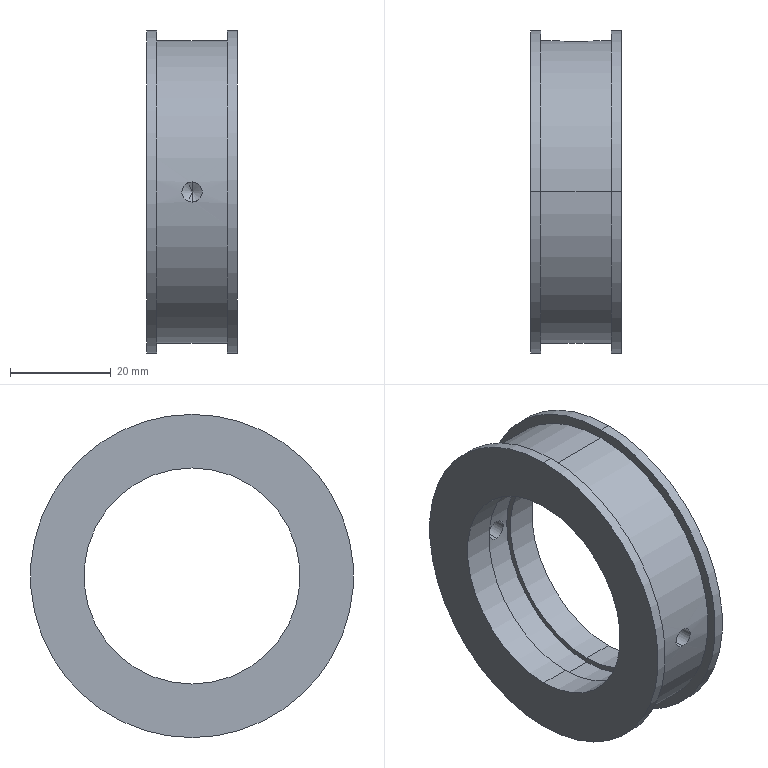Part | SolidWorks | features HoleWzd 3, Fillet 2, Revolution 1 | 1 solid | 31 faces | box 18 x 64 x 64 mm | volume 25534 mm3 | cylinder 18 | plane 7 | torus 2 | spline 2 | cone 2 | commonest cylinder face diameters 4 x4 42.8 x4 64 x4 7.5 x2 44.8 x2 60 x2
STEP:
#1=CARTESIAN_POINT('',(0.6103,28.8,3.75));
#2=VERTEX_POINT('',#1);
#3=CARTESIAN_POINT('',(0.6103,28.8,-3.75));
#4=VERTEX_POINT('',#3);
#5=CARTESIAN_POINT('',(0.6103,28.8,0.));
#6=DIRECTION('',(0.,-1.,0.));
#7=DIRECTION('',(0.,0.,-1.));
#8=AXIS2_PLACEMENT_3D('',#5,#6,#7);
#9=CIRCLE('',#8,3.75);
#10=EDGE_CURVE('',#2,#4,#9,.T.);
#11=ORIENTED_EDGE('',*,*,#10,.F.);
#12=CARTESIAN_POINT('',(0.6103,28.5,3.45));
#13=VERTEX_POINT('',#12);
#14=CARTESIAN_POINT('',(0.6103,28.8,3.45));
#15=DIRECTION('',(1.,0.,0.));
#16=DIRECTION('',(0.,0.,-1.));
#17=AXIS2_PLACEMENT_3D('',#14,#15,#16);
#18=CIRCLE('',#17,0.3);
#19=EDGE_CURVE('',#2,#13,#18,.T.);
#20=ORIENTED_EDGE('',*,*,#19,.T.);
#21=CARTESIAN_POINT('',(0.6103,28.5,-3.45));
#22=VERTEX_POINT('',#21);
#23=CARTESIAN_POINT('',(0.6103,28.5,0.));
#24=DIRECTION('',(0.,1.,0.));
#25=DIRECTION('',(0.,0.,-1.));
#26=AXIS2_PLACEMENT_3D('',#23,#24,#25);
#27=CIRCLE('',#26,3.45);
#28=EDGE_CURVE('',#22,#13,#27,.T.);
#29=ORIENTED_EDGE('',*,*,#28,.F.);
#30=CARTESIAN_POINT('',(0.6103,28.8,-3.45));
#31=DIRECTION('',(-1.,0.,0.));
#32=DIRECTION('',(0.,0.,1.));
#33=AXIS2_PLACEMENT_3D('',#30,#31,#32);
#34=CIRCLE('',#33,0.3);
#35=EDGE_CURVE('',#4,#22,#34,.T.);
#36=ORIENTED_EDGE('',*,*,#35,.F.);
#37=EDGE_LOOP('',(#11,#20,#29,#36));
#38=FACE_OUTER_BOUND('',#37,.T.);
#39=CARTESIAN_POINT('',(0.6103,28.8,0.));
#40=DIRECTION('',(0.,-1.,0.));
#41=DIRECTION('',(0.,0.,-1.));
#42=AXIS2_PLACEMENT_3D('',#39,#40,#41);
#43=TOROIDAL_SURFACE('',#42,3.45,0.3);
#44=ADVANCED_FACE('',(#38),#43,.F.);
#45=CARTESIAN_POINT('',(-0.2424,29.551,-3.652));
#46=VERTEX_POINT('',#45);
#47=CARTESIAN_POINT('',(0.6103,29.537,3.75));
#48=VERTEX_POINT('',#47);
#49=CARTESIAN_POINT('',(-0.2424,29.551,-3.652));
#50=CARTESIAN_POINT('',(-0.4646,29.558,-3.6));
#51=CARTESIAN_POINT('',(-0.6839,29.568,-3.527));
#52=CARTESIAN_POINT('',(-1.101,29.591,-3.345));
#53=CARTESIAN_POINT('',(-1.299,29.605,-3.236));
#54=CARTESIAN_POINT('',(-1.675,29.634,-2.982));
#55=CARTESIAN_POINT('',(-1.854,29.65,-2.836));
#56=CARTESIAN_POINT('',(-2.178,29.682,-2.518));
#57=CARTESIAN_POINT('',(-2.324,29.698,-2.346));
#58=CARTESIAN_POINT('',(-2.586,29.728,-1.974));
#59=CARTESIAN_POINT('',(-2.701,29.742,-1.774));
#60=CARTESIAN_POINT('',(-2.891,29.766,-1.363));
#61=CARTESIAN_POINT('',(-2.967,29.776,-1.149));
#62=CARTESIAN_POINT('',(-3.08,29.792,-0.7059));
#63=CARTESIAN_POINT('',(-3.116,29.797,-0.479));
#64=CARTESIAN_POINT('',(-3.146,29.801,-0.02683));
#65=CARTESIAN_POINT('',(-3.141,29.8,0.2003));
#66=CARTESIAN_POINT('',(-3.089,29.793,0.6567));
#67=CARTESIAN_POINT('',(-3.042,29.786,0.8794));
#68=CARTESIAN_POINT('',(-2.91,29.769,1.312));
#69=CARTESIAN_POINT('',(-2.823,29.757,1.524));
#70=CARTESIAN_POINT('',(-2.613,29.731,1.93));
#71=CARTESIAN_POINT('',(-2.491,29.717,2.121));
#72=CARTESIAN_POINT('',(-2.213,29.686,2.478));
#73=CARTESIAN_POINT('',(-2.056,29.67,2.647));
#74=CARTESIAN_POINT('',(-1.716,29.638,2.95));
#75=CARTESIAN_POINT('',(-1.534,29.623,3.084));
#76=CARTESIAN_POINT('',(-1.147,29.594,3.32));
#77=CARTESIAN_POINT('',(-0.9399,29.581,3.422));
#78=CARTESIAN_POINT('',(-0.5152,29.56,3.584));
#79=CARTESIAN_POINT('',(-0.2972,29.552,3.646));
#80=CARTESIAN_POINT('',(0.1503,29.54,3.729));
#81=CARTESIAN_POINT('',(0.3805,29.537,3.75));
#82=CARTESIAN_POINT('',(0.6103,29.537,3.75));
#83=B_SPLINE_CURVE_WITH_KNOTS('',3,(#49,#50,#51,#52,#53,#54,#55,#56,#57,#58,#59,#60,#61,#62,#63,#64,#65,#66,#67,#68,#69,#70,#71,#72,#73,#74,#75,#76,#77,#78,#79,#80,#81,#82),.UNSPECIFIED.,.F.,.F.,(4,2,2,2,2,2,2,2,2,2,2,2,2,2,2,2,4),(0.01269,0.01337,0.01406,0.01474,0.01543,0.01611,0.0168,0.01748,0.01817,0.01885,0.01954,0.02022,0.02091,0.02159,0.02228,0.02296,0.02365),.UNSPECIFIED.);
#84=EDGE_CURVE('',#46,#48,#83,.T.);
#85=ORIENTED_EDGE('',*,*,#84,.F.);
#86=CARTESIAN_POINT('',(-0.2879,29.749,-3.872));
#87=VERTEX_POINT('',#86);
#88=CARTESIAN_POINT('',(-0.2879,29.551,-3.847));
#89=DIRECTION('',(-0.9734,0.02959,0.2273));
#90=DIRECTION('',(0.2274,0.,0.9738));
#91=AXIS2_PLACEMENT_3D('',#88,#89,#90);
#92=CIRCLE('',#91,0.2);
#93=EDGE_CURVE('',#46,#87,#92,.T.);
#94=ORIENTED_EDGE('',*,*,#93,.T.);
#95=CARTESIAN_POINT('',(1.509,29.749,3.872));
#96=VERTEX_POINT('',#95);
#97=CARTESIAN_POINT('',(1.509,29.749,3.872));
#98=CARTESIAN_POINT('',(1.254,29.741,3.932));
#99=CARTESIAN_POINT('',(0.9958,29.737,3.966));
#100=CARTESIAN_POINT('',(0.4738,29.734,3.983));
#101=CARTESIAN_POINT('',(0.2098,29.737,3.965));
#102=CARTESIAN_POINT('',(-0.3023,29.748,3.878));
#103=CARTESIAN_POINT('',(-0.5513,29.757,3.81));
#104=CARTESIAN_POINT('',(-1.035,29.78,3.624));
#105=CARTESIAN_POINT('',(-1.271,29.795,3.506));
#106=CARTESIAN_POINT('',(-1.707,29.826,3.231));
#107=CARTESIAN_POINT('',(-1.911,29.843,3.072));
#108=CARTESIAN_POINT('',(-2.289,29.878,2.714));
#109=CARTESIAN_POINT('',(-2.459,29.895,2.517));
#110=CARTESIAN_POINT('',(-2.756,29.927,2.096));
#111=CARTESIAN_POINT('',(-2.886,29.943,1.869));
#112=CARTESIAN_POINT('',(-3.098,29.969,1.394));
#113=CARTESIAN_POINT('',(-3.18,29.979,1.149));
#114=CARTESIAN_POINT('',(-3.296,29.994,0.6447));
#115=CARTESIAN_POINT('',(-3.33,29.999,0.3829));
#116=CARTESIAN_POINT('',(-3.346,30.001,-0.135));
#117=CARTESIAN_POINT('',(-3.329,29.999,-0.3927));
#118=CARTESIAN_POINT('',(-3.245,29.987,-0.9056));
#119=CARTESIAN_POINT('',(-3.177,29.979,-1.16));
#120=CARTESIAN_POINT('',(-2.996,29.956,-1.643));
#121=CARTESIAN_POINT('',(-2.882,29.942,-1.876));
#122=CARTESIAN_POINT('',(-2.608,29.911,-2.321));
#123=CARTESIAN_POINT('',(-2.451,29.894,-2.526));
#124=CARTESIAN_POINT('',(-2.1,29.86,-2.904));
#125=CARTESIAN_POINT('',(-1.904,29.842,-3.078));
#126=CARTESIAN_POINT('',(-1.484,29.809,-3.382));
#127=CARTESIAN_POINT('',(-1.261,29.794,-3.512));
#128=CARTESIAN_POINT('',(-0.7903,29.768,-3.727));
#129=CARTESIAN_POINT('',(-0.5411,29.757,-3.813));
#130=CARTESIAN_POINT('',(-0.2879,29.749,-3.872));
#131=B_SPLINE_CURVE_WITH_KNOTS('',3,(#97,#98,#99,#100,#101,#102,#103,#104,#105,#106,#107,#108,#109,#110,#111,#112,#113,#114,#115,#116,#117,#118,#119,#120,#121,#122,#123,#124,#125,#126,#127,#128,#129,#130),.UNSPECIFIED.,.F.,.F.,(4,2,2,2,2,2,2,2,2,2,2,2,2,2,2,2,4),(0.02421,0.025,0.02578,0.02657,0.02735,0.02814,0.02892,0.02971,0.03049,0.03128,0.03206,0.03285,0.03363,0.03442,0.0352,0.03599,0.03677),.UNSPECIFIED.);
#132=EDGE_CURVE('',#96,#87,#131,.T.);
#133=ORIENTED_EDGE('',*,*,#132,.F.);
#134=CARTESIAN_POINT('',(1.463,29.551,3.652));
#135=VERTEX_POINT('',#134);
#136=CARTESIAN_POINT('',(1.509,29.551,3.846));
#137=DIRECTION('',(0.9734,0.02959,-0.2273));
#138=DIRECTION('',(-0.2274,0.,-0.9738));
#139=AXIS2_PLACEMENT_3D('',#136,#137,#138);
#140=CIRCLE('',#139,0.2);
#141=EDGE_CURVE('',#135,#96,#140,.T.);
#142=ORIENTED_EDGE('',*,*,#141,.F.);
#143=CARTESIAN_POINT('',(0.6103,29.537,3.75));
#144=CARTESIAN_POINT('',(0.7544,29.537,3.75));
#145=CARTESIAN_POINT('',(1.041,29.539,3.733));
#146=CARTESIAN_POINT('',(1.323,29.546,3.684));
#147=CARTESIAN_POINT('',(1.463,29.551,3.652));
#148=B_SPLINE_CURVE_WITH_KNOTS('',3,(#143,#144,#145,#146,#147),.UNSPECIFIED.,.F.,.F.,(4,1,4),(0.,0.0004293,0.0008586),.UNSPECIFIED.);
#149=EDGE_CURVE('',#48,#135,#148,.T.);
#150=ORIENTED_EDGE('',*,*,#149,.F.);
#151=EDGE_LOOP('',(#85,#94,#133,#142,#150));
#152=FACE_OUTER_BOUND('',#151,.T.);
#153=CARTESIAN_POINT('',(1.463,29.551,3.652));
#154=CARTESIAN_POINT('',(1.457,29.778,3.653));
#155=CARTESIAN_POINT('',(1.509,29.749,3.872));
#156=CARTESIAN_POINT('',(1.222,29.543,3.708));
#157=CARTESIAN_POINT('',(1.216,29.771,3.709));
#158=CARTESIAN_POINT('',(1.254,29.741,3.932));
#159=CARTESIAN_POINT('',(0.9788,29.538,3.74));
#160=CARTESIAN_POINT('',(0.9757,29.767,3.74));
#161=CARTESIAN_POINT('',(0.9985,29.737,3.966));
#162=CARTESIAN_POINT('',(0.49,29.536,3.756));
#163=CARTESIAN_POINT('',(0.4909,29.765,3.756));
#164=CARTESIAN_POINT('',(0.4835,29.734,3.983));
#165=CARTESIAN_POINT('',(0.2413,29.539,3.74));
#166=CARTESIAN_POINT('',(0.2448,29.767,3.74));
#167=CARTESIAN_POINT('',(0.2217,29.737,3.966));
#168=CARTESIAN_POINT('',(-0.2441,29.55,3.66));
#169=CARTESIAN_POINT('',(-0.237,29.777,3.661));
#170=CARTESIAN_POINT('',(-0.2896,29.748,3.881));
#171=CARTESIAN_POINT('',(-0.4801,29.558,3.596));
#172=CARTESIAN_POINT('',(-0.4712,29.784,3.599));
#173=CARTESIAN_POINT('',(-0.5383,29.757,3.814));
#174=CARTESIAN_POINT('',(-0.9391,29.581,3.424));
#175=CARTESIAN_POINT('',(-0.928,29.804,3.429));
#176=CARTESIAN_POINT('',(-1.022,29.78,3.631));
#177=CARTESIAN_POINT('',(-1.163,29.595,3.313));
#178=CARTESIAN_POINT('',(-1.151,29.817,3.32));
#179=CARTESIAN_POINT('',(-1.257,29.794,3.513));
#180=CARTESIAN_POINT('',(-1.578,29.626,3.055));
#181=CARTESIAN_POINT('',(-1.566,29.844,3.064));
#182=CARTESIAN_POINT('',(-1.695,29.825,3.24));
#183=CARTESIAN_POINT('',(-1.772,29.643,2.907));
#184=CARTESIAN_POINT('',(-1.76,29.859,2.916));
#185=CARTESIAN_POINT('',(-1.899,29.842,3.082));
#186=CARTESIAN_POINT('',(-2.132,29.677,2.57));
#187=CARTESIAN_POINT('',(-2.121,29.89,2.581));
#188=CARTESIAN_POINT('',(-2.278,29.877,2.725));
#189=CARTESIAN_POINT('',(-2.294,29.695,2.384));
#190=CARTESIAN_POINT('',(-2.285,29.905,2.396));
#191=CARTESIAN_POINT('',(-2.449,29.894,2.528));
#192=CARTESIAN_POINT('',(-2.579,29.727,1.988));
#193=CARTESIAN_POINT('',(-2.572,29.934,1.999));
#194=CARTESIAN_POINT('',(-2.749,29.927,2.108));
#195=CARTESIAN_POINT('',(-2.703,29.742,1.774));
#196=CARTESIAN_POINT('',(-2.697,29.948,1.785));
#197=CARTESIAN_POINT('',(-2.88,29.942,1.881));
#198=CARTESIAN_POINT('',(-2.907,29.768,1.325));
#199=CARTESIAN_POINT('',(-2.903,29.971,1.334));
#200=CARTESIAN_POINT('',(-3.094,29.968,1.405));
#201=CARTESIAN_POINT('',(-2.985,29.779,1.093));
#202=CARTESIAN_POINT('',(-2.983,29.981,1.101));
#203=CARTESIAN_POINT('',(-3.177,29.979,1.159));
#204=CARTESIAN_POINT('',(-3.097,29.794,0.6165));
#205=CARTESIAN_POINT('',(-3.096,29.995,0.6213));
#206=CARTESIAN_POINT('',(-3.294,29.994,0.6537));
#207=CARTESIAN_POINT('',(-3.13,29.799,0.3687));
#208=CARTESIAN_POINT('',(-3.129,29.999,0.3714));
#209=CARTESIAN_POINT('',(-3.329,29.999,0.391));
#210=CARTESIAN_POINT('',(-3.146,29.801,-0.1217));
#211=CARTESIAN_POINT('',(-3.146,30.001,-0.1225));
#212=CARTESIAN_POINT('',(-3.346,30.001,-0.129));
#213=CARTESIAN_POINT('',(-3.13,29.799,-0.3657));
#214=CARTESIAN_POINT('',(-3.13,29.999,-0.3686));
#215=CARTESIAN_POINT('',(-3.329,29.999,-0.3878));
#216=CARTESIAN_POINT('',(-3.05,29.788,-0.8512));
#217=CARTESIAN_POINT('',(-3.049,29.989,-0.8574));
#218=CARTESIAN_POINT('',(-3.245,29.988,-0.9027));
#219=CARTESIAN_POINT('',(-2.986,29.779,-1.092));
#220=CARTESIAN_POINT('',(-2.983,29.981,-1.1));
#221=CARTESIAN_POINT('',(-3.177,29.979,-1.158));
#222=CARTESIAN_POINT('',(-2.813,29.756,-1.549));
#223=CARTESIAN_POINT('',(-2.809,29.96,-1.559));
#224=CARTESIAN_POINT('',(-2.996,29.956,-1.643));
#225=CARTESIAN_POINT('',(-2.705,29.743,-1.769));
#226=CARTESIAN_POINT('',(-2.699,29.948,-1.78));
#227=CARTESIAN_POINT('',(-2.882,29.942,-1.876));
#228=CARTESIAN_POINT('',(-2.444,29.711,-2.189));
#229=CARTESIAN_POINT('',(-2.436,29.92,-2.201));
#230=CARTESIAN_POINT('',(-2.607,29.911,-2.322));
#231=CARTESIAN_POINT('',(-2.295,29.695,-2.383));
#232=CARTESIAN_POINT('',(-2.286,29.905,-2.395));
#233=CARTESIAN_POINT('',(-2.45,29.894,-2.527));
#234=CARTESIAN_POINT('',(-1.962,29.661,-2.74));
#235=CARTESIAN_POINT('',(-1.95,29.875,-2.751));
#236=CARTESIAN_POINT('',(-2.099,29.86,-2.905));
#237=CARTESIAN_POINT('',(-1.775,29.643,-2.904));
#238=CARTESIAN_POINT('',(-1.763,29.859,-2.914));
#239=CARTESIAN_POINT('',(-1.902,29.842,-3.08));
#240=CARTESIAN_POINT('',(-1.376,29.61,-3.19));
#241=CARTESIAN_POINT('',(-1.364,29.83,-3.198));
#242=CARTESIAN_POINT('',(-1.482,29.809,-3.383));
#243=CARTESIAN_POINT('',(-1.165,29.595,-3.312));
#244=CARTESIAN_POINT('',(-1.153,29.817,-3.319));
#245=CARTESIAN_POINT('',(-1.259,29.794,-3.512));
#246=CARTESIAN_POINT('',(-0.7184,29.569,-3.515));
#247=CARTESIAN_POINT('',(-0.7081,29.794,-3.519));
#248=CARTESIAN_POINT('',(-0.7893,29.768,-3.728));
#249=CARTESIAN_POINT('',(-0.4816,29.558,-3.596));
#250=CARTESIAN_POINT('',(-0.4729,29.784,-3.598));
#251=CARTESIAN_POINT('',(-0.5398,29.757,-3.813));
#252=CARTESIAN_POINT('',(-0.2424,29.551,-3.652));
#253=CARTESIAN_POINT('',(-0.2359,29.778,-3.653));
#254=CARTESIAN_POINT('',(-0.2879,29.749,-3.872));
#255=(BOUNDED_SURFACE()B_SPLINE_SURFACE(3,2,((#153,#154,#155),(#156,#157,#158),(#159,#160,#161),(#162,#163,#164),(#165,#166,#167),(#168,#169,#170),(#171,#172,#173),(#174,#175,#176),(#177,#178,#179),(#180,#181,#182),(#183,#184,#185),(#186,#187,#188),(#189,#190,#191),(#192,#193,#194),(#195,#196,#197),(#198,#199,#200),(#201,#202,#203),(#204,#205,#206),(#207,#208,#209),(#210,#211,#212),(#213,#214,#215),(#216,#217,#218),(#219,#220,#221),(#222,#223,#224),(#225,#226,#227),(#228,#229,#230),(#231,#232,#233),(#234,#235,#236),(#237,#238,#239),(#240,#241,#242),(#243,#244,#245),(#246,#247,#248),(#249,#250,#251),(#252,#253,#254)),.UNSPECIFIED.,.F.,.F.,.F.)B_SPLINE_SURFACE_WITH_KNOTS((4,2,2,2,2,2,2,2,2,2,2,2,2,2,2,2,4),(3,3),(0.,0.0007725,0.001545,0.002318,0.00309,0.003863,0.004635,0.005408,0.00618,0.006953,0.007725,0.008498,0.00927,0.01004,0.01082,0.01159,0.01236),(0.,1.),.UNSPECIFIED.)GEOMETRIC_REPRESENTATION_ITEM()RATIONAL_B_SPLINE_SURFACE(((1.,0.6612,1.),(1.,0.6597,1.),(1.,0.6588,1.),(1.,0.6584,1.),(1.,0.6589,1.),(1.,0.661,1.),(1.,0.6626,1.),(1.,0.6669,1.),(1.,0.6696,1.),(1.,0.6754,1.),(1.,0.6785,1.),(1.,0.6849,1.),(1.,0.688,1.),(1.,0.694,1.),(1.,0.6967,1.),(1.,0.7014,1.),(1.,0.7033,1.),(1.,0.706,1.),(1.,0.7069,1.),(1.,0.7073,1.),(1.,0.7069,1.),(1.,0.7049,1.),(1.,0.7033,1.),(1.,0.6992,1.),(1.,0.6968,1.),(1.,0.6911,1.),(1.,0.688,1.),(1.,0.6817,1.),(1.,0.6785,1.),(1.,0.6724,1.),(1.,0.6696,1.),(1.,0.6647,1.),(1.,0.6626,1.),(1.,0.6612,1.)))REPRESENTATION_ITEM('')SURFACE());
#256=ADVANCED_FACE('',(#152),#255,.T.);
#257=CARTESIAN_POINT('',(0.6103,-24.798,0.));
#258=VERTEX_POINT('',#257);
#259=CARTESIAN_POINT('',(0.6103,-26.,-2.));
#260=VERTEX_POINT('',#259);
#261=CARTESIAN_POINT('',(0.6103,-26.,-2.));
#262=DIRECTION('',(0.,-0.515,-0.8572));
#263=VECTOR('',#262,1000.);
#264=LINE('',#261,#263);
#265=EDGE_CURVE('',#258,#260,#264,.T.);
#266=ORIENTED_EDGE('',*,*,#265,.F.);
#267=CARTESIAN_POINT('',(0.6103,-26.,2.));
#268=VERTEX_POINT('',#267);
#269=CARTESIAN_POINT('',(0.6103,-26.,2.));
#270=DIRECTION('',(0.,-0.515,0.8572));
#271=VECTOR('',#270,1000.);
#272=LINE('',#269,#271);
#273=EDGE_CURVE('',#258,#268,#272,.T.);
#274=ORIENTED_EDGE('',*,*,#273,.T.);
#275=CARTESIAN_POINT('',(0.6103,-26.,0.));
#276=DIRECTION('',(0.,-1.,0.));
#277=DIRECTION('',(0.,0.,-1.));
#278=AXIS2_PLACEMENT_3D('',#275,#276,#277);
#279=CIRCLE('',#278,2.);
#280=EDGE_CURVE('',#268,#260,#279,.T.);
#281=ORIENTED_EDGE('',*,*,#280,.T.);
#282=EDGE_LOOP('',(#266,#274,#281));
#283=FACE_OUTER_BOUND('',#282,.T.);
#284=CARTESIAN_POINT('',(0.6103,-26.,0.));
#285=DIRECTION('',(0.,-1.,0.));
#286=DIRECTION('',(0.,0.,-1.));
#287=AXIS2_PLACEMENT_3D('',#284,#285,#286);
#288=CONICAL_SURFACE('',#287,2.,1.03);
#289=ADVANCED_FACE('',(#283),#288,.F.);
#290=ORIENTED_EDGE('',*,*,#280,.F.);
#291=CARTESIAN_POINT('',(0.6103,-29.933,2.));
#292=VERTEX_POINT('',#291);
#293=CARTESIAN_POINT('',(0.6103,-30.,2.));
#294=DIRECTION('',(0.,-1.,0.));
#295=VECTOR('',#294,1000.);
#296=LINE('',#293,#295);
#297=EDGE_CURVE('',#268,#292,#296,.T.);
#298=ORIENTED_EDGE('',*,*,#297,.T.);
#299=CARTESIAN_POINT('',(0.6103,-29.933,-2.));
#300=VERTEX_POINT('',#299);
#301=CARTESIAN_POINT('',(0.6103,-29.933,-2.));
#302=CARTESIAN_POINT('',(0.4782,-29.933,-2.));
#303=CARTESIAN_POINT('',(0.3482,-29.934,-1.987));
#304=CARTESIAN_POINT('',(0.0925,-29.937,-1.936));
#305=CARTESIAN_POINT('',(-0.03454,-29.94,-1.898));
#306=CARTESIAN_POINT('',(-0.2768,-29.946,-1.797));
#307=CARTESIAN_POINT('',(-0.3916,-29.95,-1.736));
#308=CARTESIAN_POINT('',(-0.609,-29.958,-1.591));
#309=CARTESIAN_POINT('',(-0.7119,-29.962,-1.506));
#310=CARTESIAN_POINT('',(-0.9886,-29.975,-1.229));
#311=CARTESIAN_POINT('',(-1.138,-29.984,-1.006));
#312=CARTESIAN_POINT('',(-1.337,-29.996,-0.525));
#313=CARTESIAN_POINT('',(-1.39,-30.,-0.2617));
#314=CARTESIAN_POINT('',(-1.39,-30.,0.1298));
#315=CARTESIAN_POINT('',(-1.377,-29.999,0.2623));
#316=CARTESIAN_POINT('',(-1.326,-29.996,0.5189));
#317=CARTESIAN_POINT('',(-1.288,-29.993,0.6436));
#318=CARTESIAN_POINT('',(-1.188,-29.987,0.8858));
#319=CARTESIAN_POINT('',(-1.125,-29.983,1.003));
#320=CARTESIAN_POINT('',(-0.9802,-29.975,1.22));
#321=CARTESIAN_POINT('',(-0.8975,-29.971,1.321));
#322=CARTESIAN_POINT('',(-0.7108,-29.962,1.507));
#323=CARTESIAN_POINT('',(-0.6097,-29.958,1.59));
#324=CARTESIAN_POINT('',(-0.3931,-29.95,1.735));
#325=CARTESIAN_POINT('',(-0.2762,-29.946,1.798));
#326=CARTESIAN_POINT('',(-0.03384,-29.94,1.898));
#327=CARTESIAN_POINT('',(0.09085,-29.937,1.936));
#328=CARTESIAN_POINT('',(0.3472,-29.934,1.987));
#329=CARTESIAN_POINT('',(0.4798,-29.933,2.));
#330=CARTESIAN_POINT('',(0.6103,-29.933,2.));
#331=B_SPLINE_CURVE_WITH_KNOTS('',3,(#301,#302,#303,#304,#305,#306,#307,#308,#309,#310,#311,#312,#313,#314,#315,#316,#317,#318,#319,#320,#321,#322,#323,#324,#325,#326,#327,#328,#329,#330),.UNSPECIFIED.,.F.,.F.,(4,2,2,2,2,2,2,2,2,2,2,2,2,2,4),(0.,0.0003909,0.0007818,0.001173,0.001564,0.002345,0.003127,0.003518,0.003909,0.0043,0.004691,0.005082,0.005473,0.005864,0.006255),.UNSPECIFIED.);
#332=EDGE_CURVE('',#300,#292,#331,.T.);
#333=ORIENTED_EDGE('',*,*,#332,.F.);
#334=CARTESIAN_POINT('',(0.6103,-30.,-2.));
#335=DIRECTION('',(0.,-1.,0.));
#336=VECTOR('',#335,1000.);
#337=LINE('',#334,#336);
#338=EDGE_CURVE('',#260,#300,#337,.T.);
#339=ORIENTED_EDGE('',*,*,#338,.F.);
#340=EDGE_LOOP('',(#290,#298,#333,#339));
#341=FACE_OUTER_BOUND('',#340,.T.);
#342=CARTESIAN_POINT('',(0.6103,-30.,0.));
#343=DIRECTION('',(0.,-1.,0.));
#344=DIRECTION('',(0.,0.,-1.));
#345=AXIS2_PLACEMENT_3D('',#342,#343,#344);
#346=CYLINDRICAL_SURFACE('',#345,2.);
#347=ADVANCED_FACE('',(#341),#346,.F.);
#348=CARTESIAN_POINT('',(0.6103,22.311,-2.));
#349=VERTEX_POINT('',#348);
#350=CARTESIAN_POINT('',(0.6103,22.311,2.));
#351=VERTEX_POINT('',#350);
#352=CARTESIAN_POINT('',(0.6103,22.311,-2.));
#353=CARTESIAN_POINT('',(0.3493,22.311,-2.));
#354=CARTESIAN_POINT('',(0.08608,22.315,-1.948));
#355=CARTESIAN_POINT('',(-0.3953,22.332,-1.748));
#356=CARTESIAN_POINT('',(-0.6184,22.344,-1.599));
#357=CARTESIAN_POINT('',(-0.8951,22.361,-1.323));
#358=CARTESIAN_POINT('',(-0.9796,22.367,-1.22));
#359=CARTESIAN_POINT('',(-1.125,22.378,-1.003));
#360=CARTESIAN_POINT('',(-1.186,22.383,-0.8882));
#361=CARTESIAN_POINT('',(-1.287,22.391,-0.6463));
#362=CARTESIAN_POINT('',(-1.325,22.394,-0.5192));
#363=CARTESIAN_POINT('',(-1.377,22.399,-0.2635));
#364=CARTESIAN_POINT('',(-1.39,22.4,-0.1336));
#365=CARTESIAN_POINT('',(-1.39,22.4,0.1305));
#366=CARTESIAN_POINT('',(-1.377,22.399,0.2608));
#367=CARTESIAN_POINT('',(-1.326,22.394,0.5164));
#368=CARTESIAN_POINT('',(-1.288,22.391,0.6434));
#369=CARTESIAN_POINT('',(-1.188,22.383,0.8857));
#370=CARTESIAN_POINT('',(-1.126,22.378,1.001));
#371=CARTESIAN_POINT('',(-0.9814,22.367,1.218));
#372=CARTESIAN_POINT('',(-0.897,22.361,1.321));
#373=CARTESIAN_POINT('',(-0.6206,22.344,1.598));
#374=CARTESIAN_POINT('',(-0.3977,22.332,1.747));
#375=CARTESIAN_POINT('',(0.08332,22.315,1.947));
#376=CARTESIAN_POINT('',(0.346,22.311,2.));
#377=CARTESIAN_POINT('',(0.6103,22.311,2.));
#378=B_SPLINE_CURVE_WITH_KNOTS('',3,(#352,#353,#354,#355,#356,#357,#358,#359,#360,#361,#362,#363,#364,#365,#366,#367,#368,#369,#370,#371,#372,#373,#374,#375,#376,#377),.UNSPECIFIED.,.F.,.F.,(4,2,2,2,2,2,2,2,2,2,2,2,4),(0.006256,0.007038,0.00782,0.008211,0.008601,0.008992,0.009383,0.009774,0.01017,0.01056,0.01095,0.01173,0.01251),.UNSPECIFIED.);
#379=EDGE_CURVE('',#349,#351,#378,.T.);
#380=ORIENTED_EDGE('',*,*,#379,.F.);
#381=CARTESIAN_POINT('',(0.6103,28.5,-2.));
#382=VERTEX_POINT('',#381);
#383=CARTESIAN_POINT('',(0.6103,28.5,-2.));
#384=DIRECTION('',(0.,1.,0.));
#385=VECTOR('',#384,1000.);
#386=LINE('',#383,#385);
#387=EDGE_CURVE('',#349,#382,#386,.T.);
#388=ORIENTED_EDGE('',*,*,#387,.T.);
#389=CARTESIAN_POINT('',(0.6103,28.5,2.));
#390=VERTEX_POINT('',#389);
#391=CARTESIAN_POINT('',(0.6103,28.5,0.));
#392=DIRECTION('',(0.,1.,0.));
#393=DIRECTION('',(0.,0.,1.));
#394=AXIS2_PLACEMENT_3D('',#391,#392,#393);
#395=CIRCLE('',#394,2.);
#396=EDGE_CURVE('',#382,#390,#395,.T.);
#397=ORIENTED_EDGE('',*,*,#396,.T.);
#398=CARTESIAN_POINT('',(0.6103,28.5,2.));
#399=DIRECTION('',(0.,1.,0.));
#400=VECTOR('',#399,1000.);
#401=LINE('',#398,#400);
#402=EDGE_CURVE('',#351,#390,#401,.T.);
#403=ORIENTED_EDGE('',*,*,#402,.F.);
#404=EDGE_LOOP('',(#380,#388,#397,#403));
#405=FACE_OUTER_BOUND('',#404,.T.);
#406=CARTESIAN_POINT('',(0.6103,28.5,0.));
#407=DIRECTION('',(0.,1.,0.));
#408=DIRECTION('',(0.,0.,1.));
#409=AXIS2_PLACEMENT_3D('',#406,#407,#408);
#410=CYLINDRICAL_SURFACE('',#409,2.);
#411=ADVANCED_FACE('',(#405),#410,.F.);
#412=ORIENTED_EDGE('',*,*,#10,.T.);
#413=CARTESIAN_POINT('',(0.6103,29.537,-3.75));
#414=VERTEX_POINT('',#413);
#415=CARTESIAN_POINT('',(0.6103,30.,-3.75));
#416=DIRECTION('',(0.,1.,0.));
#417=VECTOR('',#416,1000.);
#418=LINE('',#415,#417);
#419=EDGE_CURVE('',#4,#414,#418,.T.);
#420=ORIENTED_EDGE('',*,*,#419,.T.);
#421=CARTESIAN_POINT('',(0.6103,29.537,-3.75));
#422=CARTESIAN_POINT('',(0.4679,29.537,-3.75));
#423=CARTESIAN_POINT('',(0.325,29.538,-3.742));
#424=CARTESIAN_POINT('',(0.03842,29.543,-3.709));
#425=CARTESIAN_POINT('',(-0.1029,29.546,-3.684));
#426=CARTESIAN_POINT('',(-0.2424,29.551,-3.652));
#427=B_SPLINE_CURVE_WITH_KNOTS('',3,(#421,#422,#423,#424,#425,#426),.UNSPECIFIED.,.F.,.F.,(4,2,4),(0.01183,0.01226,0.01269),.UNSPECIFIED.);
#428=EDGE_CURVE('',#414,#46,#427,.T.);
#429=ORIENTED_EDGE('',*,*,#428,.T.);
#430=ORIENTED_EDGE('',*,*,#84,.T.);
#431=CARTESIAN_POINT('',(0.6103,30.,3.75));
#432=DIRECTION('',(0.,1.,0.));
#433=VECTOR('',#432,1000.);
#434=LINE('',#431,#433);
#435=EDGE_CURVE('',#2,#48,#434,.T.);
#436=ORIENTED_EDGE('',*,*,#435,.F.);
#437=EDGE_LOOP('',(#412,#420,#429,#430,#436));
#438=FACE_OUTER_BOUND('',#437,.T.);
#439=CARTESIAN_POINT('',(0.6103,30.,0.));
#440=DIRECTION('',(0.,1.,0.));
#441=DIRECTION('',(0.,0.,1.));
#442=AXIS2_PLACEMENT_3D('',#439,#440,#441);
#443=CYLINDRICAL_SURFACE('',#442,3.75);
#444=ADVANCED_FACE('',(#438),#443,.F.);
#445=CARTESIAN_POINT('',(-2.39,0.,-21.4));
#446=VERTEX_POINT('',#445);
#447=CARTESIAN_POINT('',(-2.39,0.,21.4));
#448=VERTEX_POINT('',#447);
#449=CARTESIAN_POINT('',(-2.39,0.,0.));
#450=DIRECTION('',(-1.,0.,0.));
#451=DIRECTION('',(0.,0.,1.));
#452=AXIS2_PLACEMENT_3D('',#449,#450,#451);
#453=CIRCLE('',#452,21.4);
#454=EDGE_CURVE('',#446,#448,#453,.T.);
#455=ORIENTED_EDGE('',*,*,#454,.F.);
#456=CARTESIAN_POINT('',(-8.39,0.,-21.4));
#457=VERTEX_POINT('',#456);
#458=CARTESIAN_POINT('',(-19.037,0.,-21.4));
#459=DIRECTION('',(-1.,0.,0.));
#460=VECTOR('',#459,1000.);
#461=LINE('',#458,#460);
#462=EDGE_CURVE('',#446,#457,#461,.T.);
#463=ORIENTED_EDGE('',*,*,#462,.T.);
#464=CARTESIAN_POINT('',(-8.39,0.,21.4));
#465=VERTEX_POINT('',#464);
#466=CARTESIAN_POINT('',(-8.39,0.,0.));
#467=DIRECTION('',(-1.,0.,0.));
#468=DIRECTION('',(0.,0.,1.));
#469=AXIS2_PLACEMENT_3D('',#466,#467,#468);
#470=CIRCLE('',#469,21.4);
#471=EDGE_CURVE('',#457,#465,#470,.T.);
#472=ORIENTED_EDGE('',*,*,#471,.T.);
#473=CARTESIAN_POINT('',(-19.037,0.,21.4));
#474=DIRECTION('',(-1.,0.,0.));
#475=VECTOR('',#474,1000.);
#476=LINE('',#473,#475);
#477=EDGE_CURVE('',#448,#465,#476,.T.);
#478=ORIENTED_EDGE('',*,*,#477,.F.);
#479=EDGE_LOOP('',(#455,#463,#472,#478));
#480=FACE_OUTER_BOUND('',#479,.T.);
#481=CARTESIAN_POINT('',(-19.037,0.,0.));
#482=DIRECTION('',(-1.,0.,0.));
#483=DIRECTION('',(0.,0.,1.));
#484=AXIS2_PLACEMENT_3D('',#481,#482,#483);
#485=CYLINDRICAL_SURFACE('',#484,21.4);
#486=ADVANCED_FACE('',(#480),#485,.F.);
#487=CARTESIAN_POINT('',(3.61,0.,-22.4));
#488=VERTEX_POINT('',#487);
#489=CARTESIAN_POINT('',(3.61,0.,22.4));
#490=VERTEX_POINT('',#489);
#491=CARTESIAN_POINT('',(3.61,0.,0.));
#492=DIRECTION('',(-1.,0.,0.));
#493=DIRECTION('',(0.,0.,1.));
#494=AXIS2_PLACEMENT_3D('',#491,#492,#493);
#495=CIRCLE('',#494,22.4);
#496=EDGE_CURVE('',#488,#490,#495,.T.);
#497=ORIENTED_EDGE('',*,*,#496,.F.);
#498=CARTESIAN_POINT('',(-2.39,0.,-22.4));
#499=VERTEX_POINT('',#498);
#500=CARTESIAN_POINT('',(-19.037,0.,-22.4));
#501=DIRECTION('',(-1.,0.,0.));
#502=VECTOR('',#501,1000.);
#503=LINE('',#500,#502);
#504=EDGE_CURVE('',#488,#499,#503,.T.);
#505=ORIENTED_EDGE('',*,*,#504,.T.);
#506=CARTESIAN_POINT('',(-2.39,0.,22.4));
#507=VERTEX_POINT('',#506);
#508=CARTESIAN_POINT('',(-2.39,0.,0.));
#509=DIRECTION('',(-1.,0.,0.));
#510=DIRECTION('',(0.,0.,1.));
#511=AXIS2_PLACEMENT_3D('',#508,#509,#510);
#512=CIRCLE('',#511,22.4);
#513=EDGE_CURVE('',#499,#507,#512,.T.);
#514=ORIENTED_EDGE('',*,*,#513,.T.);
#515=CARTESIAN_POINT('',(-19.037,0.,22.4));
#516=DIRECTION('',(-1.,0.,0.));
#517=VECTOR('',#516,1000.);
#518=LINE('',#515,#517);
#519=EDGE_CURVE('',#490,#507,#518,.T.);
#520=ORIENTED_EDGE('',*,*,#519,.F.);
#521=EDGE_LOOP('',(#497,#505,#514,#520));
#522=FACE_OUTER_BOUND('',#521,.T.);
#523=CARTESIAN_POINT('',(-19.037,0.,0.));
#524=DIRECTION('',(-1.,0.,0.));
#525=DIRECTION('',(0.,0.,1.));
#526=AXIS2_PLACEMENT_3D('',#523,#524,#525);
#527=CYLINDRICAL_SURFACE('',#526,22.4);
#528=ADVANCED_FACE('',(#522),#527,.F.);
#529=CARTESIAN_POINT('',(9.61,0.,-21.4));
#530=VERTEX_POINT('',#529);
#531=CARTESIAN_POINT('',(9.61,0.,21.4));
#532=VERTEX_POINT('',#531);
#533=CARTESIAN_POINT('',(9.61,0.,0.));
#534=DIRECTION('',(-1.,0.,0.));
#535=DIRECTION('',(0.,0.,1.));
#536=AXIS2_PLACEMENT_3D('',#533,#534,#535);
#537=CIRCLE('',#536,21.4);
#538=EDGE_CURVE('',#530,#532,#537,.T.);
#539=ORIENTED_EDGE('',*,*,#538,.F.);
#540=CARTESIAN_POINT('',(3.61,0.,-21.4));
#541=VERTEX_POINT('',#540);
#542=CARTESIAN_POINT('',(-19.037,0.,-21.4));
#543=DIRECTION('',(-1.,0.,0.));
#544=VECTOR('',#543,1000.);
#545=LINE('',#542,#544);
#546=EDGE_CURVE('',#530,#541,#545,.T.);
#547=ORIENTED_EDGE('',*,*,#546,.T.);
#548=CARTESIAN_POINT('',(3.61,0.,21.4));
#549=VERTEX_POINT('',#548);
#550=CARTESIAN_POINT('',(3.61,0.,0.));
#551=DIRECTION('',(-1.,0.,0.));
#552=DIRECTION('',(0.,0.,1.));
#553=AXIS2_PLACEMENT_3D('',#550,#551,#552);
#554=CIRCLE('',#553,21.4);
#555=EDGE_CURVE('',#541,#549,#554,.T.);
#556=ORIENTED_EDGE('',*,*,#555,.T.);
#557=CARTESIAN_POINT('',(-19.037,0.,21.4));
#558=DIRECTION('',(-1.,0.,0.));
#559=VECTOR('',#558,1000.);
#560=LINE('',#557,#559);
#561=EDGE_CURVE('',#532,#549,#560,.T.);
#562=ORIENTED_EDGE('',*,*,#561,.F.);
#563=EDGE_LOOP('',(#539,#547,#556,#562));
#564=FACE_OUTER_BOUND('',#563,.T.);
#565=CARTESIAN_POINT('',(-19.037,0.,0.));
#566=DIRECTION('',(-1.,0.,0.));
#567=DIRECTION('',(0.,0.,1.));
#568=AXIS2_PLACEMENT_3D('',#565,#566,#567);
#569=CYLINDRICAL_SURFACE('',#568,21.4);
#570=ADVANCED_FACE('',(#564),#569,.F.);
#571=CARTESIAN_POINT('',(9.61,0.,32.));
#572=VERTEX_POINT('',#571);
#573=CARTESIAN_POINT('',(9.61,0.,-32.));
#574=VERTEX_POINT('',#573);
#575=CARTESIAN_POINT('',(9.61,0.,0.));
#576=DIRECTION('',(-1.,0.,0.));
#577=DIRECTION('',(0.,0.,1.));
#578=AXIS2_PLACEMENT_3D('',#575,#576,#577);
#579=CIRCLE('',#578,32.);
#580=EDGE_CURVE('',#572,#574,#579,.T.);
#581=ORIENTED_EDGE('',*,*,#580,.T.);
#582=CARTESIAN_POINT('',(7.61,0.,-32.));
#583=VERTEX_POINT('',#582);
#584=CARTESIAN_POINT('',(-19.037,0.,-32.));
#585=DIRECTION('',(-1.,0.,0.));
#586=VECTOR('',#585,1000.);
#587=LINE('',#584,#586);
#588=EDGE_CURVE('',#574,#583,#587,.T.);
#589=ORIENTED_EDGE('',*,*,#588,.T.);
#590=CARTESIAN_POINT('',(7.61,0.,32.));
#591=VERTEX_POINT('',#590);
#592=CARTESIAN_POINT('',(7.61,0.,0.));
#593=DIRECTION('',(-1.,0.,0.));
#594=DIRECTION('',(0.,0.,1.));
#595=AXIS2_PLACEMENT_3D('',#592,#593,#594);
#596=CIRCLE('',#595,32.);
#597=EDGE_CURVE('',#591,#583,#596,.T.);
#598=ORIENTED_EDGE('',*,*,#597,.F.);
#599=CARTESIAN_POINT('',(-19.037,0.,32.));
#600=DIRECTION('',(-1.,0.,0.));
#601=VECTOR('',#600,1000.);
#602=LINE('',#599,#601);
#603=EDGE_CURVE('',#572,#591,#602,.T.);
#604=ORIENTED_EDGE('',*,*,#603,.F.);
#605=EDGE_LOOP('',(#581,#589,#598,#604));
#606=FACE_OUTER_BOUND('',#605,.T.);
#607=CARTESIAN_POINT('',(-19.037,0.,0.));
#608=DIRECTION('',(-1.,0.,0.));
#609=DIRECTION('',(0.,0.,1.));
#610=AXIS2_PLACEMENT_3D('',#607,#608,#609);
#611=CYLINDRICAL_SURFACE('',#610,32.);
#612=ADVANCED_FACE('',(#606),#611,.T.);
#613=ORIENTED_EDGE('',*,*,#132,.T.);
#614=CARTESIAN_POINT('',(-0.2879,29.749,-3.872));
#615=CARTESIAN_POINT('',(-0.03455,29.741,-3.932));
#616=CARTESIAN_POINT('',(0.2272,29.737,-3.966));
#617=CARTESIAN_POINT('',(0.7456,29.734,-3.983));
#618=CARTESIAN_POINT('',(1.003,29.737,-3.965));
#619=CARTESIAN_POINT('',(1.516,29.748,-3.879));
#620=CARTESIAN_POINT('',(1.77,29.757,-3.81));
#621=CARTESIAN_POINT('',(2.253,29.78,-3.626));
#622=CARTESIAN_POINT('',(2.484,29.794,-3.51));
#623=CARTESIAN_POINT('',(2.927,29.826,-3.232));
#624=CARTESIAN_POINT('',(3.131,29.843,-3.073));
#625=CARTESIAN_POINT('',(3.505,29.877,-2.718));
#626=CARTESIAN_POINT('',(3.677,29.895,-2.519));
#627=CARTESIAN_POINT('',(3.977,29.927,-2.096));
#628=CARTESIAN_POINT('',(4.105,29.942,-1.872));
#629=CARTESIAN_POINT('',(4.317,29.968,-1.399));
#630=CARTESIAN_POINT('',(4.401,29.979,-1.149));
#631=CARTESIAN_POINT('',(4.517,29.994,-0.6445));
#632=CARTESIAN_POINT('',(4.55,29.999,-0.3881));
#633=CARTESIAN_POINT('',(4.567,30.001,0.1335));
#634=CARTESIAN_POINT('',(4.549,29.998,0.3946));
#635=CARTESIAN_POINT('',(4.465,29.987,0.9045));
#636=CARTESIAN_POINT('',(4.398,29.979,1.157));
#637=CARTESIAN_POINT('',(4.216,29.956,1.646));
#638=CARTESIAN_POINT('',(4.102,29.942,1.877));
#639=CARTESIAN_POINT('',(3.831,29.911,2.317));
#640=CARTESIAN_POINT('',(3.671,29.894,2.527));
#641=CARTESIAN_POINT('',(3.319,29.86,2.906));
#642=CARTESIAN_POINT('',(3.126,29.842,3.077));
#643=CARTESIAN_POINT('',(2.705,29.809,3.381));
#644=CARTESIAN_POINT('',(2.478,29.794,3.514));
#645=CARTESIAN_POINT('',(2.008,29.768,3.728));
#646=CARTESIAN_POINT('',(1.764,29.757,3.812));
#647=CARTESIAN_POINT('',(1.509,29.749,3.872));
#648=B_SPLINE_CURVE_WITH_KNOTS('',3,(#614,#615,#616,#617,#618,#619,#620,#621,#622,#623,#624,#625,#626,#627,#628,#629,#630,#631,#632,#633,#634,#635,#636,#637,#638,#639,#640,#641,#642,#643,#644,#645,#646,#647),.UNSPECIFIED.,.F.,.F.,(4,2,2,2,2,2,2,2,2,2,2,2,2,2,2,2,4),(0.01165,0.01243,0.01322,0.014,0.01479,0.01557,0.01636,0.01714,0.01793,0.01872,0.0195,0.02029,0.02107,0.02186,0.02264,0.02343,0.02421),.UNSPECIFIED.);
#649=EDGE_CURVE('',#87,#96,#648,.T.);
#650=ORIENTED_EDGE('',*,*,#649,.T.);
#651=EDGE_LOOP('',(#613,#650));
#652=FACE_BOUND('',#651,.T.);
#653=CARTESIAN_POINT('',(7.61,0.,30.));
#654=VERTEX_POINT('',#653);
#655=CARTESIAN_POINT('',(7.61,0.,-30.));
#656=VERTEX_POINT('',#655);
#657=CARTESIAN_POINT('',(7.61,0.,0.));
#658=DIRECTION('',(-1.,0.,0.));
#659=DIRECTION('',(0.,0.,1.));
#660=AXIS2_PLACEMENT_3D('',#657,#658,#659);
#661=CIRCLE('',#660,30.);
#662=EDGE_CURVE('',#654,#656,#661,.T.);
#663=ORIENTED_EDGE('',*,*,#662,.T.);
#664=CARTESIAN_POINT('',(-6.39,0.,-30.));
#665=VERTEX_POINT('',#664);
#666=CARTESIAN_POINT('',(-19.037,0.,-30.));
#667=DIRECTION('',(-1.,0.,0.));
#668=VECTOR('',#667,1000.);
#669=LINE('',#666,#668);
#670=EDGE_CURVE('',#656,#665,#669,.T.);
#671=ORIENTED_EDGE('',*,*,#670,.T.);
#672=CARTESIAN_POINT('',(-6.39,0.,30.));
#673=VERTEX_POINT('',#672);
#674=CARTESIAN_POINT('',(-6.39,0.,0.));
#675=DIRECTION('',(-1.,0.,0.));
#676=DIRECTION('',(0.,0.,1.));
#677=AXIS2_PLACEMENT_3D('',#674,#675,#676);
#678=CIRCLE('',#677,30.);
#679=EDGE_CURVE('',#673,#665,#678,.T.);
#680=ORIENTED_EDGE('',*,*,#679,.F.);
#681=CARTESIAN_POINT('',(-19.037,0.,30.));
#682=DIRECTION('',(-1.,0.,0.));
#683=VECTOR('',#682,1000.);
#684=LINE('',#681,#683);
#685=EDGE_CURVE('',#654,#673,#684,.T.);
#686=ORIENTED_EDGE('',*,*,#685,.F.);
#687=EDGE_LOOP('',(#663,#671,#680,#686));
#688=FACE_OUTER_BOUND('',#687,.T.);
#689=CARTESIAN_POINT('',(-19.037,0.,0.));
#690=DIRECTION('',(-1.,0.,0.));
#691=DIRECTION('',(0.,0.,1.));
#692=AXIS2_PLACEMENT_3D('',#689,#690,#691);
#693=CYLINDRICAL_SURFACE('',#692,30.);
#694=ADVANCED_FACE('',(#652,#688),#693,.T.);
#695=CARTESIAN_POINT('',(-6.39,0.,32.));
#696=VERTEX_POINT('',#695);
#697=CARTESIAN_POINT('',(-6.39,0.,-32.));
#698=VERTEX_POINT('',#697);
#699=CARTESIAN_POINT('',(-6.39,0.,0.));
#700=DIRECTION('',(-1.,0.,0.));
#701=DIRECTION('',(0.,0.,1.));
#702=AXIS2_PLACEMENT_3D('',#699,#700,#701);
#703=CIRCLE('',#702,32.);
#704=EDGE_CURVE('',#696,#698,#703,.T.);
#705=ORIENTED_EDGE('',*,*,#704,.T.);
#706=CARTESIAN_POINT('',(-8.39,0.,-32.));
#707=VERTEX_POINT('',#706);
#708=CARTESIAN_POINT('',(-19.037,0.,-32.));
#709=DIRECTION('',(-1.,0.,0.));
#710=VECTOR('',#709,1000.);
#711=LINE('',#708,#710);
#712=EDGE_CURVE('',#698,#707,#711,.T.);
#713=ORIENTED_EDGE('',*,*,#712,.T.);
#714=CARTESIAN_POINT('',(-8.39,0.,32.));
#715=VERTEX_POINT('',#714);
#716=CARTESIAN_POINT('',(-8.39,0.,0.));
#717=DIRECTION('',(-1.,0.,0.));
#718=DIRECTION('',(0.,0.,1.));
#719=AXIS2_PLACEMENT_3D('',#716,#717,#718);
#720=CIRCLE('',#719,32.);
#721=EDGE_CURVE('',#715,#707,#720,.T.);
#722=ORIENTED_EDGE('',*,*,#721,.F.);
#723=CARTESIAN_POINT('',(-19.037,0.,32.));
#724=DIRECTION('',(-1.,0.,0.));
#725=VECTOR('',#724,1000.);
#726=LINE('',#723,#725);
#727=EDGE_CURVE('',#696,#715,#726,.T.);
#728=ORIENTED_EDGE('',*,*,#727,.F.);
#729=EDGE_LOOP('',(#705,#713,#722,#728));
#730=FACE_OUTER_BOUND('',#729,.T.);
#731=CARTESIAN_POINT('',(-19.037,0.,0.));
#732=DIRECTION('',(-1.,0.,0.));
#733=DIRECTION('',(0.,0.,1.));
#734=AXIS2_PLACEMENT_3D('',#731,#732,#733);
#735=CYLINDRICAL_SURFACE('',#734,32.);
#736=ADVANCED_FACE('',(#730),#735,.T.);
#737=ORIENTED_EDGE('',*,*,#712,.F.);
#738=CARTESIAN_POINT('',(-6.39,0.,0.));
#739=DIRECTION('',(-1.,0.,0.));
#740=DIRECTION('',(0.,0.,1.));
#741=AXIS2_PLACEMENT_3D('',#738,#739,#740);
#742=CIRCLE('',#741,32.);
#743=EDGE_CURVE('',#698,#696,#742,.T.);
#744=ORIENTED_EDGE('',*,*,#743,.T.);
#745=ORIENTED_EDGE('',*,*,#727,.T.);
#746=CARTESIAN_POINT('',(-8.39,0.,0.));
#747=DIRECTION('',(-1.,0.,0.));
#748=DIRECTION('',(0.,0.,1.));
#749=AXIS2_PLACEMENT_3D('',#746,#747,#748);
#750=CIRCLE('',#749,32.);
#751=EDGE_CURVE('',#707,#715,#750,.T.);
#752=ORIENTED_EDGE('',*,*,#751,.F.);
#753=EDGE_LOOP('',(#737,#744,#745,#752));
#754=FACE_OUTER_BOUND('',#753,.T.);
#755=CARTESIAN_POINT('',(-19.037,0.,0.));
#756=DIRECTION('',(-1.,0.,0.));
#757=DIRECTION('',(0.,0.,1.));
#758=AXIS2_PLACEMENT_3D('',#755,#756,#757);
#759=CYLINDRICAL_SURFACE('',#758,32.);
#760=ADVANCED_FACE('',(#754),#759,.T.);
#761=ORIENTED_EDGE('',*,*,#704,.F.);
#762=ORIENTED_EDGE('',*,*,#743,.F.);
#763=EDGE_LOOP('',(#761,#762));
#764=FACE_OUTER_BOUND('',#763,.T.);
#765=ORIENTED_EDGE('',*,*,#679,.T.);
#766=CARTESIAN_POINT('',(-6.39,0.,0.));
#767=DIRECTION('',(-1.,0.,0.));
#768=DIRECTION('',(0.,0.,1.));
#769=AXIS2_PLACEMENT_3D('',#766,#767,#768);
#770=CIRCLE('',#769,30.);
#771=EDGE_CURVE('',#665,#673,#770,.T.);
#772=ORIENTED_EDGE('',*,*,#771,.T.);
#773=EDGE_LOOP('',(#765,#772));
#774=FACE_BOUND('',#773,.T.);
#775=CARTESIAN_POINT('',(-6.39,32.,0.));
#776=DIRECTION('',(-1.,0.,0.));
#777=DIRECTION('',(0.,0.,1.));
#778=AXIS2_PLACEMENT_3D('',#775,#776,#777);
#779=PLANE('',#778);
#780=ADVANCED_FACE('',(#764,#774),#779,.F.);
#781=ORIENTED_EDGE('',*,*,#670,.F.);
#782=CARTESIAN_POINT('',(7.61,0.,0.));
#783=DIRECTION('',(-1.,0.,0.));
#784=DIRECTION('',(0.,0.,1.));
#785=AXIS2_PLACEMENT_3D('',#782,#783,#784);
#786=CIRCLE('',#785,30.);
#787=EDGE_CURVE('',#656,#654,#786,.T.);
#788=ORIENTED_EDGE('',*,*,#787,.T.);
#789=ORIENTED_EDGE('',*,*,#685,.T.);
#790=ORIENTED_EDGE('',*,*,#771,.F.);
#791=EDGE_LOOP('',(#781,#788,#789,#790));
#792=FACE_OUTER_BOUND('',#791,.T.);
#793=ORIENTED_EDGE('',*,*,#332,.T.);
#794=CARTESIAN_POINT('',(0.6103,-29.933,2.));
#795=CARTESIAN_POINT('',(0.8714,-29.933,2.));
#796=CARTESIAN_POINT('',(1.135,-29.937,1.948));
#797=CARTESIAN_POINT('',(1.616,-29.949,1.748));
#798=CARTESIAN_POINT('',(1.839,-29.958,1.599));
#799=CARTESIAN_POINT('',(2.116,-29.971,1.323));
#800=CARTESIAN_POINT('',(2.2,-29.975,1.22));
#801=CARTESIAN_POINT('',(2.346,-29.983,1.003));
#802=CARTESIAN_POINT('',(2.407,-29.987,0.8881));
#803=CARTESIAN_POINT('',(2.508,-29.993,0.6462));
#804=CARTESIAN_POINT('',(2.546,-29.996,0.5191));
#805=CARTESIAN_POINT('',(2.597,-29.999,0.2635));
#806=CARTESIAN_POINT('',(2.61,-30.,0.1336));
#807=CARTESIAN_POINT('',(2.61,-30.,-0.1304));
#808=CARTESIAN_POINT('',(2.598,-29.999,-0.2607));
#809=CARTESIAN_POINT('',(2.547,-29.996,-0.5163));
#810=CARTESIAN_POINT('',(2.509,-29.993,-0.6432));
#811=CARTESIAN_POINT('',(2.408,-29.987,-0.8857));
#812=CARTESIAN_POINT('',(2.347,-29.984,-1.001));
#813=CARTESIAN_POINT('',(2.202,-29.975,-1.218));
#814=CARTESIAN_POINT('',(2.118,-29.971,-1.321));
#815=CARTESIAN_POINT('',(1.933,-29.962,-1.506));
#816=CARTESIAN_POINT('',(1.833,-29.958,-1.588));
#817=CARTESIAN_POINT('',(1.615,-29.95,-1.735));
#818=CARTESIAN_POINT('',(1.498,-29.946,-1.797));
#819=CARTESIAN_POINT('',(1.137,-29.937,-1.947));
#820=CARTESIAN_POINT('',(0.8746,-29.933,-2.));
#821=CARTESIAN_POINT('',(0.6103,-29.933,-2.));
#822=B_SPLINE_CURVE_WITH_KNOTS('',3,(#794,#795,#796,#797,#798,#799,#800,#801,#802,#803,#804,#805,#806,#807,#808,#809,#810,#811,#812,#813,#814,#815,#816,#817,#818,#819,#820,#821),.UNSPECIFIED.,.F.,.F.,(4,2,2,2,2,2,2,2,2,2,2,2,2,4),(0.006255,0.007036,0.007818,0.008209,0.0086,0.00899,0.009381,0.009772,0.01016,0.01055,0.01094,0.01134,0.01173,0.01251),.UNSPECIFIED.);
#823=EDGE_CURVE('',#292,#300,#822,.T.);
#824=ORIENTED_EDGE('',*,*,#823,.T.);
#825=EDGE_LOOP('',(#793,#824));
#826=FACE_BOUND('',#825,.T.);
#827=CARTESIAN_POINT('',(-19.037,0.,0.));
#828=DIRECTION('',(-1.,0.,0.));
#829=DIRECTION('',(0.,0.,1.));
#830=AXIS2_PLACEMENT_3D('',#827,#828,#829);
#831=CYLINDRICAL_SURFACE('',#830,30.);
#832=ADVANCED_FACE('',(#792,#826),#831,.T.);
#833=ORIENTED_EDGE('',*,*,#662,.F.);
#834=ORIENTED_EDGE('',*,*,#787,.F.);
#835=EDGE_LOOP('',(#833,#834));
#836=FACE_BOUND('',#835,.T.);
#837=ORIENTED_EDGE('',*,*,#597,.T.);
#838=CARTESIAN_POINT('',(7.61,0.,0.));
#839=DIRECTION('',(-1.,0.,0.));
#840=DIRECTION('',(0.,0.,1.));
#841=AXIS2_PLACEMENT_3D('',#838,#839,#840);
#842=CIRCLE('',#841,32.);
#843=EDGE_CURVE('',#583,#591,#842,.T.);
#844=ORIENTED_EDGE('',*,*,#843,.T.);
#845=EDGE_LOOP('',(#837,#844));
#846=FACE_OUTER_BOUND('',#845,.T.);
#847=CARTESIAN_POINT('',(7.61,30.,0.));
#848=DIRECTION('',(1.,0.,0.));
#849=DIRECTION('',(0.,0.,-1.));
#850=AXIS2_PLACEMENT_3D('',#847,#848,#849);
#851=PLANE('',#850);
#852=ADVANCED_FACE('',(#836,#846),#851,.F.);
#853=ORIENTED_EDGE('',*,*,#588,.F.);
#854=CARTESIAN_POINT('',(9.61,0.,0.));
#855=DIRECTION('',(-1.,0.,0.));
#856=DIRECTION('',(0.,0.,1.));
#857=AXIS2_PLACEMENT_3D('',#854,#855,#856);
#858=CIRCLE('',#857,32.);
#859=EDGE_CURVE('',#574,#572,#858,.T.);
#860=ORIENTED_EDGE('',*,*,#859,.T.);
#861=ORIENTED_EDGE('',*,*,#603,.T.);
#862=ORIENTED_EDGE('',*,*,#843,.F.);
#863=EDGE_LOOP('',(#853,#860,#861,#862));
#864=FACE_OUTER_BOUND('',#863,.T.);
#865=CARTESIAN_POINT('',(-19.037,0.,0.));
#866=DIRECTION('',(-1.,0.,0.));
#867=DIRECTION('',(0.,0.,1.));
#868=AXIS2_PLACEMENT_3D('',#865,#866,#867);
#869=CYLINDRICAL_SURFACE('',#868,32.);
#870=ADVANCED_FACE('',(#864),#869,.T.);
#871=ORIENTED_EDGE('',*,*,#580,.F.);
#872=ORIENTED_EDGE('',*,*,#859,.F.);
#873=EDGE_LOOP('',(#871,#872));
#874=FACE_OUTER_BOUND('',#873,.T.);
#875=CARTESIAN_POINT('',(9.61,0.,0.));
#876=DIRECTION('',(-1.,0.,0.));
#877=DIRECTION('',(0.,0.,1.));
#878=AXIS2_PLACEMENT_3D('',#875,#876,#877);
#879=CIRCLE('',#878,21.4);
#880=EDGE_CURVE('',#532,#530,#879,.T.);
#881=ORIENTED_EDGE('',*,*,#880,.T.);
#882=ORIENTED_EDGE('',*,*,#538,.T.);
#883=EDGE_LOOP('',(#881,#882));
#884=FACE_BOUND('',#883,.T.);
#885=CARTESIAN_POINT('',(9.61,32.,0.));
#886=DIRECTION('',(-1.,0.,0.));
#887=DIRECTION('',(0.,0.,1.));
#888=AXIS2_PLACEMENT_3D('',#885,#886,#887);
#889=PLANE('',#888);
#890=ADVANCED_FACE('',(#874,#884),#889,.F.);
#891=ORIENTED_EDGE('',*,*,#546,.F.);
#892=ORIENTED_EDGE('',*,*,#880,.F.);
#893=ORIENTED_EDGE('',*,*,#561,.T.);
#894=CARTESIAN_POINT('',(3.61,0.,0.));
#895=DIRECTION('',(-1.,0.,0.));
#896=DIRECTION('',(0.,0.,1.));
#897=AXIS2_PLACEMENT_3D('',#894,#895,#896);
#898=CIRCLE('',#897,21.4);
#899=EDGE_CURVE('',#549,#541,#898,.T.);
#900=ORIENTED_EDGE('',*,*,#899,.T.);
#901=EDGE_LOOP('',(#891,#892,#893,#900));
#902=FACE_OUTER_BOUND('',#901,.T.);
#903=CARTESIAN_POINT('',(-19.037,0.,0.));
#904=DIRECTION('',(-1.,0.,0.));
#905=DIRECTION('',(0.,0.,1.));
#906=AXIS2_PLACEMENT_3D('',#903,#904,#905);
#907=CYLINDRICAL_SURFACE('',#906,21.4);
#908=ADVANCED_FACE('',(#902),#907,.F.);
#909=ORIENTED_EDGE('',*,*,#899,.F.);
#910=ORIENTED_EDGE('',*,*,#555,.F.);
#911=EDGE_LOOP('',(#909,#910));
#912=FACE_BOUND('',#911,.T.);
#913=CARTESIAN_POINT('',(3.61,0.,0.));
#914=DIRECTION('',(-1.,0.,0.));
#915=DIRECTION('',(0.,0.,1.));
#916=AXIS2_PLACEMENT_3D('',#913,#914,#915);
#917=CIRCLE('',#916,22.4);
#918=EDGE_CURVE('',#490,#488,#917,.T.);
#919=ORIENTED_EDGE('',*,*,#918,.T.);
#920=ORIENTED_EDGE('',*,*,#496,.T.);
#921=EDGE_LOOP('',(#919,#920));
#922=FACE_OUTER_BOUND('',#921,.T.);
#923=CARTESIAN_POINT('',(3.61,21.4,0.));
#924=DIRECTION('',(1.,0.,0.));
#925=DIRECTION('',(0.,0.,-1.));
#926=AXIS2_PLACEMENT_3D('',#923,#924,#925);
#927=PLANE('',#926);
#928=ADVANCED_FACE('',(#912,#922),#927,.F.);
#929=ORIENTED_EDGE('',*,*,#504,.F.);
#930=ORIENTED_EDGE('',*,*,#918,.F.);
#931=ORIENTED_EDGE('',*,*,#519,.T.);
#932=CARTESIAN_POINT('',(-2.39,0.,0.));
#933=DIRECTION('',(-1.,0.,0.));
#934=DIRECTION('',(0.,0.,1.));
#935=AXIS2_PLACEMENT_3D('',#932,#933,#934);
#936=CIRCLE('',#935,22.4);
#937=EDGE_CURVE('',#507,#499,#936,.T.);
#938=ORIENTED_EDGE('',*,*,#937,.T.);
#939=EDGE_LOOP('',(#929,#930,#931,#938));
#940=FACE_OUTER_BOUND('',#939,.T.);
#941=CARTESIAN_POINT('',(0.6103,22.311,2.));
#942=CARTESIAN_POINT('',(0.7426,22.311,2.));
#943=CARTESIAN_POINT('',(0.8725,22.312,1.987));
#944=CARTESIAN_POINT('',(1.128,22.316,1.936));
#945=CARTESIAN_POINT('',(1.255,22.32,1.898));
#946=CARTESIAN_POINT('',(1.498,22.328,1.797));
#947=CARTESIAN_POINT('',(1.612,22.333,1.736));
#948=CARTESIAN_POINT('',(1.83,22.344,1.591));
#949=CARTESIAN_POINT('',(1.933,22.349,1.506));
#950=CARTESIAN_POINT('',(2.209,22.367,1.229));
#951=CARTESIAN_POINT('',(2.358,22.379,1.006));
#952=CARTESIAN_POINT('',(2.558,22.395,0.5251));
#953=CARTESIAN_POINT('',(2.61,22.4,0.2618));
#954=CARTESIAN_POINT('',(2.61,22.4,-0.1298));
#955=CARTESIAN_POINT('',(2.597,22.399,-0.2624));
#956=CARTESIAN_POINT('',(2.546,22.394,-0.5189));
#957=CARTESIAN_POINT('',(2.508,22.391,-0.6437));
#958=CARTESIAN_POINT('',(2.408,22.383,-0.8859));
#959=CARTESIAN_POINT('',(2.346,22.378,-1.003));
#960=CARTESIAN_POINT('',(2.201,22.367,-1.22));
#961=CARTESIAN_POINT('',(2.118,22.361,-1.321));
#962=CARTESIAN_POINT('',(1.931,22.349,-1.507));
#963=CARTESIAN_POINT('',(1.83,22.344,-1.59));
#964=CARTESIAN_POINT('',(1.614,22.333,-1.735));
#965=CARTESIAN_POINT('',(1.497,22.328,-1.798));
#966=CARTESIAN_POINT('',(1.255,22.32,-1.898));
#967=CARTESIAN_POINT('',(1.13,22.316,-1.936));
#968=CARTESIAN_POINT('',(0.8735,22.312,-1.987));
#969=CARTESIAN_POINT('',(0.7409,22.311,-2.));
#970=CARTESIAN_POINT('',(0.6103,22.311,-2.));
#971=B_SPLINE_CURVE_WITH_KNOTS('',3,(#941,#942,#943,#944,#945,#946,#947,#948,#949,#950,#951,#952,#953,#954,#955,#956,#957,#958,#959,#960,#961,#962,#963,#964,#965,#966,#967,#968,#969,#970),.UNSPECIFIED.,.F.,.F.,(4,2,2,2,2,2,2,2,2,2,2,2,2,2,4),(0.,0.000391,0.000782,0.001173,0.001564,0.002346,0.003128,0.003519,0.00391,0.004301,0.004692,0.005083,0.005474,0.005865,0.006256),.UNSPECIFIED.);
#972=EDGE_CURVE('',#351,#349,#971,.T.);
#973=ORIENTED_EDGE('',*,*,#972,.T.);
#974=ORIENTED_EDGE('',*,*,#379,.T.);
#975=EDGE_LOOP('',(#973,#974));
#976=FACE_BOUND('',#975,.T.);
#977=CARTESIAN_POINT('',(-19.037,0.,0.));
#978=DIRECTION('',(-1.,0.,0.));
#979=DIRECTION('',(0.,0.,1.));
#980=AXIS2_PLACEMENT_3D('',#977,#978,#979);
#981=CYLINDRICAL_SURFACE('',#980,22.4);
#982=ADVANCED_FACE('',(#940,#976),#981,.F.);
#983=ORIENTED_EDGE('',*,*,#937,.F.);
#984=ORIENTED_EDGE('',*,*,#513,.F.);
#985=EDGE_LOOP('',(#983,#984));
#986=FACE_OUTER_BOUND('',#985,.T.);
#987=CARTESIAN_POINT('',(-2.39,0.,0.));
#988=DIRECTION('',(-1.,0.,0.));
#989=DIRECTION('',(0.,0.,1.));
#990=AXIS2_PLACEMENT_3D('',#987,#988,#989);
#991=CIRCLE('',#990,21.4);
#992=EDGE_CURVE('',#448,#446,#991,.T.);
#993=ORIENTED_EDGE('',*,*,#992,.T.);
#994=ORIENTED_EDGE('',*,*,#454,.T.);
#995=EDGE_LOOP('',(#993,#994));
#996=FACE_BOUND('',#995,.T.);
#997=CARTESIAN_POINT('',(-2.39,22.4,0.));
#998=DIRECTION('',(-1.,0.,0.));
#999=DIRECTION('',(0.,0.,1.));
#1000=AXIS2_PLACEMENT_3D('',#997,#998,#999);
#1001=PLANE('',#1000);
#1002=ADVANCED_FACE('',(#986,#996),#1001,.F.);
#1003=ORIENTED_EDGE('',*,*,#462,.F.);
#1004=ORIENTED_EDGE('',*,*,#992,.F.);
#1005=ORIENTED_EDGE('',*,*,#477,.T.);
#1006=CARTESIAN_POINT('',(-8.39,0.,0.));
#1007=DIRECTION('',(-1.,0.,0.));
#1008=DIRECTION('',(0.,0.,1.));
#1009=AXIS2_PLACEMENT_3D('',#1006,#1007,#1008);
#1010=CIRCLE('',#1009,21.4);
#1011=EDGE_CURVE('',#465,#457,#1010,.T.);
#1012=ORIENTED_EDGE('',*,*,#1011,.T.);
#1013=EDGE_LOOP('',(#1003,#1004,#1005,#1012));
#1014=FACE_OUTER_BOUND('',#1013,.T.);
#1015=CARTESIAN_POINT('',(-19.037,0.,0.));
#1016=DIRECTION('',(-1.,0.,0.));
#1017=DIRECTION('',(0.,0.,1.));
#1018=AXIS2_PLACEMENT_3D('',#1015,#1016,#1017);
#1019=CYLINDRICAL_SURFACE('',#1018,21.4);
#1020=ADVANCED_FACE('',(#1014),#1019,.F.);
#1021=ORIENTED_EDGE('',*,*,#1011,.F.);
#1022=ORIENTED_EDGE('',*,*,#471,.F.);
#1023=EDGE_LOOP('',(#1021,#1022));
#1024=FACE_BOUND('',#1023,.T.);
#1025=ORIENTED_EDGE('',*,*,#721,.T.);
#1026=ORIENTED_EDGE('',*,*,#751,.T.);
#1027=EDGE_LOOP('',(#1025,#1026));
#1028=FACE_OUTER_BOUND('',#1027,.T.);
#1029=CARTESIAN_POINT('',(-8.39,21.4,0.));
#1030=DIRECTION('',(1.,0.,0.));
#1031=DIRECTION('',(0.,0.,-1.));
#1032=AXIS2_PLACEMENT_3D('',#1029,#1030,#1031);
#1033=PLANE('',#1032);
#1034=ADVANCED_FACE('',(#1024,#1028),#1033,.F.);
#1035=ORIENTED_EDGE('',*,*,#419,.F.);
#1036=CARTESIAN_POINT('',(0.6103,28.8,0.));
#1037=DIRECTION('',(0.,-1.,0.));
#1038=DIRECTION('',(0.,0.,-1.));
#1039=AXIS2_PLACEMENT_3D('',#1036,#1037,#1038);
#1040=CIRCLE('',#1039,3.75);
#1041=EDGE_CURVE('',#4,#2,#1040,.T.);
#1042=ORIENTED_EDGE('',*,*,#1041,.T.);
#1043=ORIENTED_EDGE('',*,*,#435,.T.);
#1044=ORIENTED_EDGE('',*,*,#149,.T.);
#1045=CARTESIAN_POINT('',(1.463,29.551,3.652));
#1046=CARTESIAN_POINT('',(1.687,29.558,3.599));
#1047=CARTESIAN_POINT('',(1.903,29.568,3.528));
#1048=CARTESIAN_POINT('',(2.318,29.591,3.346));
#1049=CARTESIAN_POINT('',(2.519,29.605,3.236));
#1050=CARTESIAN_POINT('',(2.898,29.634,2.981));
#1051=CARTESIAN_POINT('',(3.073,29.65,2.837));
#1052=CARTESIAN_POINT('',(3.396,29.682,2.52));
#1053=CARTESIAN_POINT('',(3.546,29.698,2.345));
#1054=CARTESIAN_POINT('',(3.808,29.728,1.972));
#1055=CARTESIAN_POINT('',(3.921,29.742,1.776));
#1056=CARTESIAN_POINT('',(4.111,29.766,1.364));
#1057=CARTESIAN_POINT('',(4.188,29.776,1.146));
#1058=CARTESIAN_POINT('',(4.301,29.792,0.7048));
#1059=CARTESIAN_POINT('',(4.336,29.797,0.4809));
#1060=CARTESIAN_POINT('',(4.367,29.801,0.02634));
#1061=CARTESIAN_POINT('',(4.362,29.8,-0.2052));
#1062=CARTESIAN_POINT('',(4.309,29.793,-0.6562));
#1063=CARTESIAN_POINT('',(4.263,29.787,-0.8782));
#1064=CARTESIAN_POINT('',(4.13,29.769,-1.315));
#1065=CARTESIAN_POINT('',(4.042,29.757,-1.528));
#1066=CARTESIAN_POINT('',(3.834,29.731,-1.93));
#1067=CARTESIAN_POINT('',(3.711,29.717,-2.121));
#1068=CARTESIAN_POINT('',(3.431,29.686,-2.482));
#1069=CARTESIAN_POINT('',(3.274,29.67,-2.649));
#1070=CARTESIAN_POINT('',(2.937,29.638,-2.95));
#1071=CARTESIAN_POINT('',(2.754,29.622,-3.086));
#1072=CARTESIAN_POINT('',(2.362,29.594,-3.324));
#1073=CARTESIAN_POINT('',(2.158,29.581,-3.423));
#1074=CARTESIAN_POINT('',(1.735,29.56,-3.585));
#1075=CARTESIAN_POINT('',(1.513,29.551,-3.647));
#1076=CARTESIAN_POINT('',(1.063,29.54,-3.73));
#1077=CARTESIAN_POINT('',(0.8374,29.537,-3.75));
#1078=CARTESIAN_POINT('',(0.6103,29.537,-3.75));
#1079=B_SPLINE_CURVE_WITH_KNOTS('',3,(#1045,#1046,#1047,#1048,#1049,#1050,#1051,#1052,#1053,#1054,#1055,#1056,#1057,#1058,#1059,#1060,#1061,#1062,#1063,#1064,#1065,#1066,#1067,#1068,#1069,#1070,#1071,#1072,#1073,#1074,#1075,#1076,#1077,#1078),.UNSPECIFIED.,.F.,.F.,(4,2,2,2,2,2,2,2,2,2,2,2,2,2,2,2,4),(0.0008586,0.001544,0.00223,0.002915,0.0036,0.004286,0.004971,0.005657,0.006342,0.007028,0.007713,0.008399,0.009084,0.00977,0.01046,0.01114,0.01183),.UNSPECIFIED.);
#1080=EDGE_CURVE('',#135,#414,#1079,.T.);
#1081=ORIENTED_EDGE('',*,*,#1080,.T.);
#1082=EDGE_LOOP('',(#1035,#1042,#1043,#1044,#1081));
#1083=FACE_OUTER_BOUND('',#1082,.T.);
#1084=CARTESIAN_POINT('',(0.6103,30.,0.));
#1085=DIRECTION('',(0.,1.,0.));
#1086=DIRECTION('',(0.,0.,1.));
#1087=AXIS2_PLACEMENT_3D('',#1084,#1085,#1086);
#1088=CYLINDRICAL_SURFACE('',#1087,3.75);
#1089=ADVANCED_FACE('',(#1083),#1088,.F.);
#1090=ORIENTED_EDGE('',*,*,#28,.T.);
#1091=CARTESIAN_POINT('',(0.6103,28.5,0.));
#1092=DIRECTION('',(0.,1.,0.));
#1093=DIRECTION('',(0.,0.,-1.));
#1094=AXIS2_PLACEMENT_3D('',#1091,#1092,#1093);
#1095=CIRCLE('',#1094,3.45);
#1096=EDGE_CURVE('',#13,#22,#1095,.T.);
#1097=ORIENTED_EDGE('',*,*,#1096,.T.);
#1098=EDGE_LOOP('',(#1090,#1097));
#1099=FACE_OUTER_BOUND('',#1098,.T.);
#1100=CARTESIAN_POINT('',(0.6103,28.5,0.));
#1101=DIRECTION('',(0.,1.,0.));
#1102=DIRECTION('',(0.,0.,1.));
#1103=AXIS2_PLACEMENT_3D('',#1100,#1101,#1102);
#1104=CIRCLE('',#1103,2.);
#1105=EDGE_CURVE('',#390,#382,#1104,.T.);
#1106=ORIENTED_EDGE('',*,*,#1105,.F.);
#1107=ORIENTED_EDGE('',*,*,#396,.F.);
#1108=EDGE_LOOP('',(#1106,#1107));
#1109=FACE_BOUND('',#1108,.T.);
#1110=CARTESIAN_POINT('',(0.6103,28.5,0.));
#1111=DIRECTION('',(0.,-1.,0.));
#1112=DIRECTION('',(0.,0.,-1.));
#1113=AXIS2_PLACEMENT_3D('',#1110,#1111,#1112);
#1114=PLANE('',#1113);
#1115=ADVANCED_FACE('',(#1099,#1109),#1114,.F.);
#1116=ORIENTED_EDGE('',*,*,#387,.F.);
#1117=ORIENTED_EDGE('',*,*,#972,.F.);
#1118=ORIENTED_EDGE('',*,*,#402,.T.);
#1119=ORIENTED_EDGE('',*,*,#1105,.T.);
#1120=EDGE_LOOP('',(#1116,#1117,#1118,#1119));
#1121=FACE_OUTER_BOUND('',#1120,.T.);
#1122=CARTESIAN_POINT('',(0.6103,28.5,0.));
#1123=DIRECTION('',(0.,1.,0.));
#1124=DIRECTION('',(0.,0.,1.));
#1125=AXIS2_PLACEMENT_3D('',#1122,#1123,#1124);
#1126=CYLINDRICAL_SURFACE('',#1125,2.);
#1127=ADVANCED_FACE('',(#1121),#1126,.F.);
#1128=ORIENTED_EDGE('',*,*,#297,.F.);
#1129=CARTESIAN_POINT('',(0.6103,-26.,0.));
#1130=DIRECTION('',(0.,-1.,0.));
#1131=DIRECTION('',(0.,0.,-1.));
#1132=AXIS2_PLACEMENT_3D('',#1129,#1130,#1131);
#1133=CIRCLE('',#1132,2.);
#1134=EDGE_CURVE('',#260,#268,#1133,.T.);
#1135=ORIENTED_EDGE('',*,*,#1134,.F.);
#1136=ORIENTED_EDGE('',*,*,#338,.T.);
#1137=ORIENTED_EDGE('',*,*,#823,.F.);
#1138=EDGE_LOOP('',(#1128,#1135,#1136,#1137));
#1139=FACE_OUTER_BOUND('',#1138,.T.);
#1140=CARTESIAN_POINT('',(0.6103,-30.,0.));
#1141=DIRECTION('',(0.,-1.,0.));
#1142=DIRECTION('',(0.,0.,-1.));
#1143=AXIS2_PLACEMENT_3D('',#1140,#1141,#1142);
#1144=CYLINDRICAL_SURFACE('',#1143,2.);
#1145=ADVANCED_FACE('',(#1139),#1144,.F.);
#1146=ORIENTED_EDGE('',*,*,#273,.F.);
#1147=ORIENTED_EDGE('',*,*,#265,.T.);
#1148=ORIENTED_EDGE('',*,*,#1134,.T.);
#1149=EDGE_LOOP('',(#1146,#1147,#1148));
#1150=FACE_OUTER_BOUND('',#1149,.T.);
#1151=CARTESIAN_POINT('',(0.6103,-26.,0.));
#1152=DIRECTION('',(0.,-1.,0.));
#1153=DIRECTION('',(0.,0.,-1.));
#1154=AXIS2_PLACEMENT_3D('',#1151,#1152,#1153);
#1155=CONICAL_SURFACE('',#1154,2.,1.03);
#1156=ADVANCED_FACE('',(#1150),#1155,.F.);
#1157=ORIENTED_EDGE('',*,*,#93,.F.);
#1158=ORIENTED_EDGE('',*,*,#428,.F.);
#1159=ORIENTED_EDGE('',*,*,#1080,.F.);
#1160=ORIENTED_EDGE('',*,*,#141,.T.);
#1161=ORIENTED_EDGE('',*,*,#649,.F.);
#1162=EDGE_LOOP('',(#1157,#1158,#1159,#1160,#1161));
#1163=FACE_OUTER_BOUND('',#1162,.T.);
#1164=CARTESIAN_POINT('',(-0.2424,29.551,-3.652));
#1165=CARTESIAN_POINT('',(-0.2359,29.778,-3.653));
#1166=CARTESIAN_POINT('',(-0.2879,29.749,-3.872));
#1167=CARTESIAN_POINT('',(-0.003271,29.543,-3.708));
#1168=CARTESIAN_POINT('',(0.002191,29.771,-3.708));
#1169=CARTESIAN_POINT('',(-0.036,29.741,-3.932));
#1170=CARTESIAN_POINT('',(0.245,29.538,-3.74));
#1171=CARTESIAN_POINT('',(0.248,29.767,-3.74));
#1172=CARTESIAN_POINT('',(0.2255,29.737,-3.966));
#1173=CARTESIAN_POINT('',(0.7356,29.536,-3.756));
#1174=CARTESIAN_POINT('',(0.7346,29.765,-3.756));
#1175=CARTESIAN_POINT('',(0.7422,29.734,-3.983));
#1176=CARTESIAN_POINT('',(0.9795,29.539,-3.74));
#1177=CARTESIAN_POINT('',(0.9761,29.767,-3.74));
#1178=CARTESIAN_POINT('',(0.9992,29.737,-3.966));
#1179=CARTESIAN_POINT('',(1.465,29.55,-3.66));
#1180=CARTESIAN_POINT('',(1.458,29.777,-3.661));
#1181=CARTESIAN_POINT('',(1.51,29.748,-3.881));
#1182=CARTESIAN_POINT('',(1.705,29.559,-3.595));
#1183=CARTESIAN_POINT('',(1.696,29.784,-3.598));
#1184=CARTESIAN_POINT('',(1.764,29.757,-3.812));
#1185=CARTESIAN_POINT('',(2.163,29.581,-3.422));
#1186=CARTESIAN_POINT('',(2.152,29.804,-3.427));
#1187=CARTESIAN_POINT('',(2.245,29.78,-3.629));
#1188=CARTESIAN_POINT('',(2.382,29.595,-3.314));
#1189=CARTESIAN_POINT('',(2.37,29.817,-3.321));
#1190=CARTESIAN_POINT('',(2.477,29.794,-3.514));
#1191=CARTESIAN_POINT('',(2.803,29.626,-3.053));
#1192=CARTESIAN_POINT('',(2.79,29.844,-3.061));
#1193=CARTESIAN_POINT('',(2.919,29.825,-3.237));
#1194=CARTESIAN_POINT('',(2.996,29.643,-2.903));
#1195=CARTESIAN_POINT('',(2.984,29.859,-2.913));
#1196=CARTESIAN_POINT('',(3.124,29.842,-3.079));
#1197=CARTESIAN_POINT('',(3.353,29.677,-2.57));
#1198=CARTESIAN_POINT('',(3.342,29.89,-2.581));
#1199=CARTESIAN_POINT('',(3.499,29.877,-2.725));
#1200=CARTESIAN_POINT('',(3.517,29.695,-2.383));
#1201=CARTESIAN_POINT('',(3.507,29.905,-2.394));
#1202=CARTESIAN_POINT('',(3.672,29.894,-2.527));
#1203=CARTESIAN_POINT('',(3.802,29.727,-1.983));
#1204=CARTESIAN_POINT('',(3.795,29.934,-1.995));
#1205=CARTESIAN_POINT('',(3.973,29.927,-2.103));
#1206=CARTESIAN_POINT('',(3.924,29.742,-1.772));
#1207=CARTESIAN_POINT('',(3.919,29.948,-1.783));
#1208=CARTESIAN_POINT('',(4.101,29.942,-1.879));
#1209=CARTESIAN_POINT('',(4.127,29.768,-1.326));
#1210=CARTESIAN_POINT('',(4.123,29.971,-1.335));
#1211=CARTESIAN_POINT('',(4.314,29.968,-1.406));
#1212=CARTESIAN_POINT('',(4.207,29.779,-1.089));
#1213=CARTESIAN_POINT('',(4.205,29.981,-1.097));
#1214=CARTESIAN_POINT('',(4.399,29.979,-1.155));
#1215=CARTESIAN_POINT('',(4.318,29.794,-0.6125));
#1216=CARTESIAN_POINT('',(4.317,29.995,-0.6172));
#1217=CARTESIAN_POINT('',(4.516,29.994,-0.6494));
#1218=CARTESIAN_POINT('',(4.35,29.799,-0.37));
#1219=CARTESIAN_POINT('',(4.35,29.999,-0.3726));
#1220=CARTESIAN_POINT('',(4.55,29.999,-0.3923));
#1221=CARTESIAN_POINT('',(4.366,29.801,0.1235));
#1222=CARTESIAN_POINT('',(4.367,30.001,0.1243));
#1223=CARTESIAN_POINT('',(4.567,30.001,0.131));
#1224=CARTESIAN_POINT('',(4.35,29.799,0.3706));
#1225=CARTESIAN_POINT('',(4.35,29.999,0.3736));
#1226=CARTESIAN_POINT('',(4.549,29.999,0.393));
#1227=CARTESIAN_POINT('',(4.27,29.788,0.8529));
#1228=CARTESIAN_POINT('',(4.269,29.989,0.8591));
#1229=CARTESIAN_POINT('',(4.465,29.987,0.9045));
#1230=CARTESIAN_POINT('',(4.206,29.779,1.092));
#1231=CARTESIAN_POINT('',(4.204,29.981,1.1));
#1232=CARTESIAN_POINT('',(4.398,29.979,1.158));
#1233=CARTESIAN_POINT('',(4.032,29.756,1.554));
#1234=CARTESIAN_POINT('',(4.028,29.96,1.564));
#1235=CARTESIAN_POINT('',(4.215,29.956,1.647));
#1236=CARTESIAN_POINT('',(3.924,29.742,1.773));
#1237=CARTESIAN_POINT('',(3.918,29.948,1.784));
#1238=CARTESIAN_POINT('',(4.101,29.942,1.88));
#1239=CARTESIAN_POINT('',(3.666,29.712,2.188));
#1240=CARTESIAN_POINT('',(3.657,29.92,2.2));
#1241=CARTESIAN_POINT('',(3.829,29.911,2.32));
#1242=CARTESIAN_POINT('',(3.514,29.694,2.386));
#1243=CARTESIAN_POINT('',(3.504,29.905,2.397));
#1244=CARTESIAN_POINT('',(3.669,29.894,2.53));
#1245=CARTESIAN_POINT('',(3.179,29.66,2.743));
#1246=CARTESIAN_POINT('',(3.168,29.874,2.754));
#1247=CARTESIAN_POINT('',(3.316,29.859,2.909));
#1248=CARTESIAN_POINT('',(2.996,29.643,2.904));
#1249=CARTESIAN_POINT('',(2.984,29.859,2.914));
#1250=CARTESIAN_POINT('',(3.123,29.842,3.079));
#1251=CARTESIAN_POINT('',(2.597,29.61,3.19));
#1252=CARTESIAN_POINT('',(2.584,29.83,3.198));
#1253=CARTESIAN_POINT('',(2.702,29.809,3.383));
#1254=CARTESIAN_POINT('',(2.381,29.595,3.315));
#1255=CARTESIAN_POINT('',(2.369,29.816,3.321));
#1256=CARTESIAN_POINT('',(2.476,29.794,3.515));
#1257=CARTESIAN_POINT('',(1.936,29.569,3.516));
#1258=CARTESIAN_POINT('',(1.926,29.794,3.52));
#1259=CARTESIAN_POINT('',(2.007,29.768,3.729));
#1260=CARTESIAN_POINT('',(1.705,29.558,3.595));
#1261=CARTESIAN_POINT('',(1.696,29.784,3.598));
#1262=CARTESIAN_POINT('',(1.763,29.757,3.813));
#1263=CARTESIAN_POINT('',(1.463,29.551,3.652));
#1264=CARTESIAN_POINT('',(1.457,29.778,3.653));
#1265=CARTESIAN_POINT('',(1.509,29.749,3.872));
#1266=(BOUNDED_SURFACE()B_SPLINE_SURFACE(3,2,((#1164,#1165,#1166),(#1167,#1168,#1169),(#1170,#1171,#1172),(#1173,#1174,#1175),(#1176,#1177,#1178),(#1179,#1180,#1181),(#1182,#1183,#1184),(#1185,#1186,#1187),(#1188,#1189,#1190),(#1191,#1192,#1193),(#1194,#1195,#1196),(#1197,#1198,#1199),(#1200,#1201,#1202),(#1203,#1204,#1205),(#1206,#1207,#1208),(#1209,#1210,#1211),(#1212,#1213,#1214),(#1215,#1216,#1217),(#1218,#1219,#1220),(#1221,#1222,#1223),(#1224,#1225,#1226),(#1227,#1228,#1229),(#1230,#1231,#1232),(#1233,#1234,#1235),(#1236,#1237,#1238),(#1239,#1240,#1241),(#1242,#1243,#1244),(#1245,#1246,#1247),(#1248,#1249,#1250),(#1251,#1252,#1253),(#1254,#1255,#1256),(#1257,#1258,#1259),(#1260,#1261,#1262),(#1263,#1264,#1265)),.UNSPECIFIED.,.F.,.F.,.F.)B_SPLINE_SURFACE_WITH_KNOTS((4,2,2,2,2,2,2,2,2,2,2,2,2,2,2,2,4),(3,3),(0.01236,0.01313,0.01391,0.01468,0.01545,0.01622,0.017,0.01777,0.01854,0.01931,0.02009,0.02086,0.02163,0.0224,0.02318,0.02395,0.02472),(0.,1.),.UNSPECIFIED.)GEOMETRIC_REPRESENTATION_ITEM()RATIONAL_B_SPLINE_SURFACE(((1.,0.6612,1.),(1.,0.6597,1.),(1.,0.6588,1.),(1.,0.6584,1.),(1.,0.6589,1.),(1.,0.661,1.),(1.,0.6627,1.),(1.,0.667,1.),(1.,0.6696,1.),(1.,0.6754,1.),(1.,0.6785,1.),(1.,0.6849,1.),(1.,0.6881,1.),(1.,0.694,1.),(1.,0.6967,1.),(1.,0.7014,1.),(1.,0.7033,1.),(1.,0.706,1.),(1.,0.7069,1.),(1.,0.7073,1.),(1.,0.7068,1.),(1.,0.7049,1.),(1.,0.7033,1.),(1.,0.6992,1.),(1.,0.6967,1.),(1.,0.6911,1.),(1.,0.688,1.),(1.,0.6817,1.),(1.,0.6785,1.),(1.,0.6724,1.),(1.,0.6695,1.),(1.,0.6647,1.),(1.,0.6626,1.),(1.,0.6612,1.)))REPRESENTATION_ITEM('')SURFACE());
#1267=ADVANCED_FACE('',(#1163),#1266,.T.);
#1268=ORIENTED_EDGE('',*,*,#19,.F.);
#1269=ORIENTED_EDGE('',*,*,#1041,.F.);
#1270=ORIENTED_EDGE('',*,*,#35,.T.);
#1271=ORIENTED_EDGE('',*,*,#1096,.F.);
#1272=EDGE_LOOP('',(#1268,#1269,#1270,#1271));
#1273=FACE_OUTER_BOUND('',#1272,.T.);
#1274=CARTESIAN_POINT('',(0.6103,28.8,0.));
#1275=DIRECTION('',(0.,-1.,0.));
#1276=DIRECTION('',(0.,0.,-1.));
#1277=AXIS2_PLACEMENT_3D('',#1274,#1275,#1276);
#1278=TOROIDAL_SURFACE('',#1277,3.45,0.3);
#1279=ADVANCED_FACE('',(#1273),#1278,.F.);
#1280=CLOSED_SHELL('',(#44,#256,#289,#347,#411,#444,#486,#528,#570,#612,#694,#736,#760,#780,#832,#852,#870,#890,#908,#928,#982,#1002,#1020,#1034,#1089,#1115,#1127,#1145,#1156,#1267,#1279));
#1281=MANIFOLD_SOLID_BREP('',#1280);
#1282=CARTESIAN_POINT('',(0.,0.,0.));
#1283=DIRECTION('',(0.,0.,1.));
#1284=DIRECTION('',(1.,0.,0.));
#1285=AXIS2_PLACEMENT_3D('',#1282,#1283,#1284);
#1286=(LENGTH_UNIT()NAMED_UNIT(*)SI_UNIT(.MILLI.,.METRE.));
#1287=UNCERTAINTY_MEASURE_WITH_UNIT(LENGTH_MEASURE(0.00001),#1286,'','');
#1288=(NAMED_UNIT(*)PLANE_ANGLE_UNIT()SI_UNIT($,.RADIAN.));
#1289=(NAMED_UNIT(*)SI_UNIT($,.STERADIAN.)SOLID_ANGLE_UNIT());
#1290=(GEOMETRIC_REPRESENTATION_CONTEXT(3)GLOBAL_UNCERTAINTY_ASSIGNED_CONTEXT((#1287))GLOBAL_UNIT_ASSIGNED_CONTEXT((#1286,#1288,#1289))REPRESENTATION_CONTEXT('',''));
#1291=ADVANCED_BREP_SHAPE_REPRESENTATION('',(#1281,#1285),#1290);